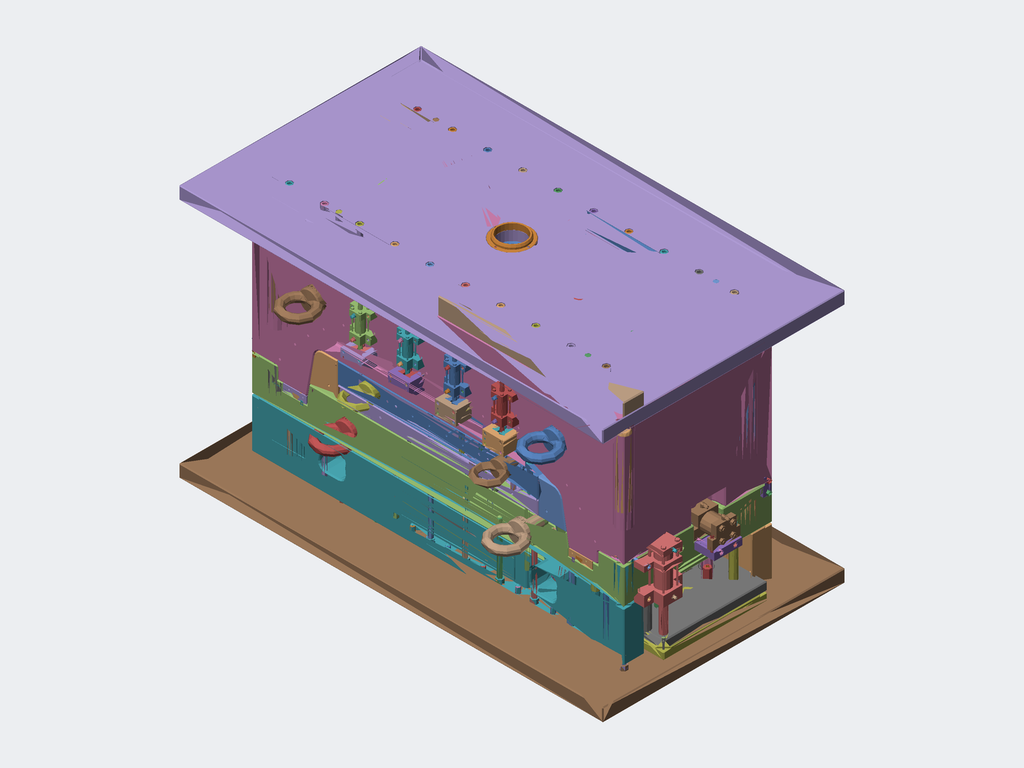Assembly | STEP file | 249 different items | 1127 placed
Parts list (item | name | quantity | parent item | size | volume):
1 | solid 1 | x44 | in A3 | 16 x 16 x 65 mm | 6021 mm3
2 | solid 10 | x4 | in A3 | 40 x 40 x 100 mm | 109109 mm3
3 | solid 100 | x2 | in A3 | 141 x 24 x 24 mm | 30892 mm3
4 | solid 101 | x4 | in A3 | 18 x 18 x 82 mm | 10396 mm3
5 | solid 102 | x1 | in A3 | 80 x 100 x 40 mm | 232410 mm3
6 | solid 103 | x1 | in A3 | 10 x 24 x 10 mm | 907.17 mm3
7 | solid 104 | x2 | in A3 | 30 x 112.165 x 452.721 mm | 308363 mm3
8 | solid 105 | x1 | in A3 | 169 x 36 x 36 mm | 85875 mm3
9 | solid 106 | x1 | in A3 | 2450 x 1400 x 75.5 mm | 255795045 mm3
10 | solid 107 | x1 | in A3 | 1075 x 120 x 100 mm | 12371190 mm3
11 | solid 108 | x1 | in A3 | 1075 x 120.001 x 100 mm | 10949894 mm3
12 | solid 109 | x20 | in A3 | 36 x 36 x 209.5 mm | 104197 mm3
13 | solid 11 | x4 | in A3 | 40 x 40 x 100 mm | 109109 mm3
14 | solid 110 | x4 | in A3 | 30 x 30 x 140 mm | 98871 mm3
15 | solid 111 | x1 | in A3 | 14.856 x 17.662 x 17.662 mm | 2886 mm3
16 | solid 112 | x1 | in A3 | 14.856 x 17.662 x 17.662 mm | 2886 mm3
17 | solid 113 | x3 | in A3 | 15.066 x 16.653 x 17.055 mm | 1616 mm3
18 | solid 114 | x2 | in A3 | 18.126 x 15.123 x 18.251 mm | 1616 mm3
19 | solid 115 | x4 | in A3 | 16 x 16 x 38 mm | 3900 mm3
20 | solid 116 | x1 | in A3 | 100 x 25.292 x 82.969 mm | 104423 mm3
21 | solid 117 | x6 | in A3 | 23.471 x 100 x 70 mm | 88768 mm3
22 | solid 118 | x2 | in A3 | 64.193 x 74.193 x 40 mm | 137435 mm3
23 | solid 119 | x16 | in A3 | 16 x 16 x 54 mm | 5157 mm3
24 | solid 12 | x20 | in A3 | 36 x 36 x 324 mm | 155996 mm3
25 | solid 120 | x1 | in A3 | 25 x 36.961 x 150.435 mm | 48566 mm3
26 | solid 121 | x1 | in A3 | 20 x 20 x 674.011 mm | 136324 mm3
27 | solid 122 | x1 | in A3 | - | 271064204 mm3
28 | solid 123 | x1 | in A3 | 25 x 36.961 x 150.435 mm | 48566 mm3
29 | solid 124 | x2 | in A3 | 120 x 30.646 x 121.053 mm | 166220 mm3
30 | solid 125 | x1 | in A3 | 20 x 20 x 674.011 mm | 136325 mm3
31 | solid 126 | x1 | in A3 | 275.799 x 860 x 518.917 mm | 54222779 mm3
32 | solid 127 | x1 | in A3 | 215.526 x 420.609 x 290.404 mm | 6486474 mm3
33 | solid 128 | x1 | in A3 | 1159 x 120 x 150 mm | 11583265 mm3
34 | solid 129 | x12 | in A3 | 36 x 36 x 114 mm | 60994 mm3
35 | solid 13 | x2 | in A3 | 98 x 98 x 290 mm | 2182712 mm3
36 | solid 130 | x2 | in A3 | 100 x 100 x 80 mm | 601369 mm3
37 | solid 131 | x2 | in A3 | 24 x 24 x 103 mm | 23254 mm3
38 | solid 132 | x4 | in A3 | 45 x 45 x 440 mm | 555891 mm3
39 | solid 133 | x24 | in A3 | 34 x 17 x 19.63 mm | 5633 mm3
40 | solid 134 | x4 | in A3 | 81 x 24 x 24 mm | 18829 mm3
41 | solid 135 | x1 | in A3 | 115 x 220 x 470 mm | 3142718 mm3
42 | solid 136 | x4 | in A3 | 18 x 18 x 77 mm | 9833 mm3
43 | solid 137 | x4 | in A3 | 40 x 40 x 60 mm | 64101 mm3
44 | solid 138 | x8 | in A3 | 36 x 36 x 154 mm | 79089 mm3
45 | solid 139 | x1 | in A3 | 169 x 36 x 36 mm | 85875 mm3
46 | solid 14 | x5 | in A3 | 18 x 18 x 67 mm | 8702 mm3
47 | solid 140 | x1 | in A3 | 119 x 36 x 36 mm | 63256 mm3
48 | solid 141 | x2 | in A3 | 166 x 236 x 100.5 mm | 770612 mm3
49 | solid 142 | x2 | in A3 | 166 x 236 x 100.5 mm | 770612 mm3
50 | solid 143 | x4 | in A3 | 70 x 60 x 80 mm | 220295 mm3
51 | solid 144 | x2 | in A3 | 120 x 90 x 80 mm | 514851 mm3
52 | solid 145 | x4 | in A3 | 25 x 214.479 x 25 mm | 62211 mm3
53 | solid 146 | x4 | in A3 | 10 x 100 x 10 mm | 7854 mm3
54 | solid 147 | x8 | in A3 | 16 x 50 x 16 mm | 4838 mm3
55 | solid 148 | x1 | in A3 | 120 x 70 x 261 mm | 645284 mm3
56 | solid 149 | x4 | in A3 | 16 x 120 x 16 mm | 24127 mm3
57 | solid 15 | x1 | in A3 | 2450 x 1400 x 75.5 mm | 249798342 mm3
58 | solid 150 | x4 | in A3 | 25 x 210.948 x 25 mm | 49531 mm3
59 | solid 151 | x1 | in A3 | 335.969 x 60 x 260.545 mm | 1623800 mm3
60 | solid 152 | x2 | in A3 | 400.456 x 100 x 296.842 mm | 2354176 mm3
61 | solid 153 | x1 | in A3 | 191.822 x 70 x 220.454 mm | 648426 mm3
62 | solid 154 | x2 | in A3 | 25 x 212.652 x 25 mm | 69526 mm3
63 | solid 155 | x2 | in A3 | 25 x 214.101 x 25 mm | 62890 mm3
64 | solid 156 | x4 | in A3 | 18 x 57 x 18 mm | 7569 mm3
65 | solid 157 | x2 | in A3 | 209.196 x 80 x 256.267 mm | 975283 mm3
66 | solid 158 | x6 | in A3 | 33.249 x 33.249 x 28.575 mm | 19000 mm3
67 | solid 159 | x5 | in A3 | 33.249 x 33.249 x 28.575 mm | 19000 mm3
68 | solid 16 | x37 | in A3 | 17.662 x 14.856 x 17.662 mm | 2886 mm3
69 | solid 160 | x1 | in A3 | 30.5 x 1 x 274.425 mm | 8203 mm3
70 | solid 161 | x6 | in A3 | 30.5 x 30.5 x 309.163 mm | 221417 mm3
71 | solid 162 | x1 | in A3 | 30.5 x 1 x 214.425 mm | 6372 mm3
72 | solid 163 | x1 | in A3 | 30.5 x 1 x 159.425 mm | 4694 mm3
73 | solid 164 | x1 | in A3 | 30.5 x 1 x 144.425 mm | 4236 mm3
74 | solid 165 | x1 | in A3 | 30.5 x 1 x 134.425 mm | 3931 mm3
75 | solid 166 | x1 | in A3 | 30.5 x 1 x 129.425 mm | 3778 mm3
76 | solid 167 | x12 | in A3 | 33.249 x 33.249 x 28.575 mm | 19000 mm3
77 | solid 168 | x5 | in A3 | 33.249 x 33.249 x 28.575 mm | 19000 mm3
78 | solid 169 | x4 | in A3 | 15 x 240 x 15 mm | 42412 mm3
79 | solid 17 | x8 | in A3 | 28.401 x 28.401 x 2.4 mm | 543.953 mm3
80 | solid 170 | x16 | in A3 | 16 x 50 x 16 mm | 4838 mm3
81 | solid 171 | x2 | in A3 | 120 x 70 x 281 mm | 651567 mm3
82 | solid 172 | x4 | in A3 | 10 x 10 x 21 mm | 822.37 mm3
83 | solid 173 | x5 | in A3 | 30 x 30 x 13 mm | 8174 mm3
84 | solid 174 | x4 | in A3 | 16 x 16 x 30 mm | 6011 mm3
85 | solid 175 | x4 | in A3 | 30 x 30 x 10 mm | 4966 mm3
86 | solid 176 | x4 | in A3 | 18 x 57 x 18 mm | 7569 mm3
87 | solid 177 | x2 | in A3 | 120 x 70 x 271 mm | 648426 mm3
88 | solid 178 | x8 | in A3 | 16 x 50 x 16 mm | 4838 mm3
89 | solid 179 | x1 | in A3 | 120 x 70 x 261 mm | 645284 mm3
90 | solid 18 | x5 | in A3 | 36 x 36 x 119 mm | 63256 mm3
91 | solid 180 | x1 | in A3 | 191.822 x 70 x 220.454 mm | 648426 mm3
92 | solid 181 | x1 | in A3 | 166.33 x 90 x 157.702 mm | 730851 mm3
93 | solid 182 | x1 | in A3 | 335.969 x 60 x 260.545 mm | 1623800 mm3
94 | solid 183 | x16 | in A3 | 16 x 104.2 x 16 mm | 9078 mm3
95 | solid 184 | x4 | in A3 | 70 x 60 x 80 mm | 220295 mm3
96 | solid 185 | x4 | in A3 | 120 x 90 x 80 mm | 514851 mm3
97 | solid 186 | x1 | in A3 | 78 x 78 x 172.328 mm | 163780 mm3
98 | solid 187 | x2 | in A3 | 25 x 204.048 x 25 mm | 59820 mm3
99 | solid 188 | x2 | in A3 | 25 x 209.468 x 25 mm | 61087 mm3
100 | solid 189 | x1 | in A3 | 78 x 78 x 380.197 mm | 321503 mm3
101 | solid 19 | x2 | in A3 | 13 x 13 x 31 mm | 2077 mm3
102 | solid 190 | x18 | in A3 | 33.249 x 33.249 x 28.575 mm | 19000 mm3
103 | solid 191 | x18 | in A3 | 33.249 x 33.249 x 28.575 mm | 19000 mm3
104 | solid 192 | x1 | in A3 | 33.249 x 33.249 x 28.575 mm | 19000 mm3
105 | solid 193 | x2 | in A3 | 102 x 14 x 16.166 mm | 8632 mm3
106 | solid 194 | x4 | in A3 | 81 x 24 x 24 mm | 18829 mm3
107 | solid 195 | x10 | in A3 | 13 x 13 x 103 mm | 5695 mm3
108 | solid 196 | x2 | in A3 | 28.652 x 26.452 x 20 mm | 5174 mm3
109 | solid 197 | x2 | in A3 | 26.803 x 29.047 x 24 mm | 6695 mm3
110 | solid 198 | x2 | in A3 | 78 x 78 x 475.57 mm | 368550 mm3
111 | solid 199 | x4 | in A3 | 12.786 x 19.739 x 20 mm | 475.009 mm3
112 | solid 2 | x2 | in A3 | 98 x 98 x 290 mm | 2182712 mm3
113 | solid 20 | x2 | in A3 | 99.984 x 40 x 48.51 mm | 156692 mm3
114 | solid 200 | x2 | in A3 | 28.652 x 26.452 x 20 mm | 5174 mm3
115 | solid 201 | x2 | in A3 | 26.803 x 29.047 x 24 mm | 6695 mm3
116 | solid 202 | x2 | in A3 | 13 x 13 x 98 mm | 5444 mm3
117 | solid 203 | x1 | in A3 | 10 x 24 x 10 mm | 907.171 mm3
118 | solid 204 | x2 | in A3 | 141 x 24 x 24 mm | 30892 mm3
119 | solid 205 | x1 | in A3 | 115 x 160 x 40 mm | 667851 mm3
120 | solid 206 | x1 | in A3 | 320.319 x 160 x 137.691 mm | 2188170 mm3
121 | solid 207 | x4 | in A3 | 42 x 42 x 12 mm | 15756 mm3
122 | solid 208 | x4 | in A3 | 10 x 10 x 21 mm | 822.719 mm3
123 | solid 209 | x12 | in A3 | 10 x 10 x 19 mm | 766.17 mm3
124 | solid 21 | x9 | in A3 | 17.662 x 17.662 x 14.856 mm | 2886 mm3
125 | solid 210 | x4 | in A3 | 125 x 125 x 10 mm | 67442 mm3
126 | solid 211 | x4 | in A3 | 95 x 95 x 120 mm | 243778 mm3
127 | solid 212 | x1 | in A3 | 2150 x 860 x 210.001 mm | 305924028 mm3
128 | solid 213 | x1 | in A3 | 115 x 220 x 470 mm | 3142718 mm3
129 | solid 214 | x2 | in A3 | 45 x 52.5 x 46 mm | 85031 mm3
130 | solid 215 | x2 | in A3 | 68 x 24 x 24 mm | 16217 mm3
131 | solid 216 | x2 | in A3 | 70 x 65 x 18 mm | 70637 mm3
132 | solid 217 | x2 | in A3 | 120 x 65 x 18 mm | 129137 mm3
133 | solid 218 | x1 | in A3 | 10 x 24 x 10 mm | 907.171 mm3
134 | solid 219 | x2 | in A3 | 15 x 15 x 25 mm | 4386 mm3
135 | solid 22 | x2 | in A3 | 121.532 x 24.876 x 80 mm | 116975 mm3
136 | solid 220 | x1 | in A3 | 10 x 24 x 10 mm | 907.17 mm3
137 | solid 221 | x3 | in A3 | 30 x 73.163 x 849.352 mm | 585466 mm3
138 | solid 222 | x4 | in A3 | 101 x 100 x 60 mm | 261945 mm3
139 | solid 223 | x8 | in A3 | 30 x 30 x 30 mm | 9761 mm3
140 | solid 224 | x1 | in A3 | 645.466 x 105.916 x 113.789 mm | 5298019 mm3
141 | solid 225 | x1 | in A3 | 80 x 100 x 40 mm | 232410 mm3
142 | solid 226 | x1 | in A3 | 2350 x 620 x 50 mm | 60712018 mm3
143 | solid 227 | x1 | in A3 | 2350 x 620 x 50 mm | 65620843 mm3
144 | solid 228 | x1 | in A3 | 2150 x 120 x 290 mm | 66813400 mm3
145 | solid 229 | x1 | in A3 | 2150 x 120 x 290 mm | 67733928 mm3
146 | solid 23 | x1 | in A3 | 135.51 x 264.332 x 188.118 mm | 3455186 mm3
147 | solid 230 | x4 | in A3 | 13 x 13 x 26 mm | 1825 mm3
148 | solid 231 | x1 | in A3 | 175 x 175 x 20 mm | 232149 mm3
149 | solid 232 | x1 | in A3 | 210 x 210 x 35 mm | 357720 mm3
150 | solid 233 | x1 | in A3 | 1344 x 458.517 x 80 mm | 15931765 mm3
151 | solid 234 | x1 | in A3 | 10 x 10 x 21 mm | 822.37 mm3
152 | solid 235 | x4 | in A3 | 13 x 13 x 103 mm | 5695 mm3
153 | solid 236 | x2 | in A3 | 22 x 22 x 728.65 mm | 268884 mm3
154 | solid 237 | x1 | in A3 | 1075 x 120 x 100 mm | 12067312 mm3
155 | solid 238 | x1 | in A3 | 1075 x 120 x 100 mm | 10949620 mm3
156 | solid 239 | x1 | in A3 | 1159 x 120 x 150 mm | 11582986 mm3
157 | solid 24 | x6 | in A3 | 14.157 x 12.856 x 14.157 mm | 1616 mm3
158 | solid 240 | x2 | in A3 | 22 x 22 x 730.955 mm | 269760 mm3
159 | solid 241 | x1 | in A3 | 74.217 x 43.029 x 40.25 mm | 106174 mm3
160 | solid 242 | x2 | in A3 | 74.238 x 44.192 x 40.9 mm | 109549 mm3
161 | solid 243 | x1 | in A3 | 74.214 x 43.098 x 40.392 mm | 106427 mm3
162 | solid 244 | x2 | in A3 | 94.183 x 59.188 x 39.916 mm | 147837 mm3
163 | solid 245 | x1 | in A3 | 35 x 46.15 x 148.499 mm | 104448 mm3
164 | solid 246 | x2 | in A3 | 40 x 85.054 x 24 mm | 60155 mm3
165 | solid 247 | x1 | in A3 | 35 x 46.15 x 148.499 mm | 104448 mm3
166 | solid 248 | x1 | in A3 | 819.765 x 65.53 x 111.578 mm | 4185351 mm3
167 | solid 249 | x1 | in A3 | - | -
168 | solid 25 | x8 | in A3 | 14.157 x 12.856 x 14.157 mm | 1616 mm3
169 | solid 26 | x1 | in A3 | 135.51 x 264.332 x 188.118 mm | 3455192 mm3
170 | solid 27 | x2 | in A3 | 11.3 x 11.3 x 16.5 mm | 595.104 mm3
171 | solid 28 | x2 | in A3 | 32 x 32 x 8 mm | 5898 mm3
172 | solid 29 | x2 | in A3 | 35 x 35 x 965 mm | 683981 mm3
173 | solid 3 | x4 | in A3 | 24 x 24 x 86.5 mm | 19937 mm3
174 | solid 30 | x12 | in A3 | 10 x 110 x 10 mm | 8639 mm3
175 | solid 31 | x8 | in A3 | 16 x 104.2 x 16 mm | 9078 mm3
176 | solid 32 | x1 | in A3 | 166.33 x 90 x 157.702 mm | 730851 mm3
177 | solid 33 | x8 | in A3 | 16 x 104.2 x 16 mm | 9078 mm3
178 | solid 34 | x2 | in A3 | 25.029 x 60 x 25.037 mm | 10130 mm3
179 | solid 35 | x3 | in A3 | 25.029 x 50 x 25.037 mm | 8248 mm3
180 | solid 36 | x2 | in A3 | 56 x 24 x 24 mm | 13802 mm3
181 | solid 37 | x2 | in A3 | 15 x 50 x 100 mm | 66748 mm3
182 | solid 38 | x2 | in A3 | 56 x 24 x 24 mm | 13802 mm3
183 | solid 39 | x4 | in A3 | 70 x 70 x 435 mm | 1546175 mm3
184 | solid 4 | x4 | in A3 | 50 x 50 x 360 mm | 617922 mm3
185 | solid 40 | x4 | in A3 | 90 x 90 x 422 mm | 2099670 mm3
186 | solid 41 | x1 | in A3 | 164.037 x 503.365 x 295.607 mm | 9582610 mm3
187 | solid 42 | x1 | in A3 | 164.037 x 503.365 x 295.607 mm | 9580661 mm3
188 | solid 43 | x1 | in A3 | - | -
189 | solid 44 | x4 | in A3 | 206 x 298 x 120.501 mm | 1511005 mm3
190 | solid 45 | x4 | in A3 | 206 x 298 x 120.501 mm | 1511009 mm3
191 | solid 46 | x1 | in A3 | - | 211233 mm3
192 | solid 47 | x2 | in A3 | 32 x 32 x 30 mm | 9356 mm3
193 | solid 48 | x1 | in A3 | 25 x 25 x 917.392 mm | 438618 mm3
194 | solid 49 | x4 | in A3 | 100 x 100 x 100 mm | 753638 mm3
195 | solid 5 | x4 | in A3 | 70 x 70 x 100 mm | 136102 mm3
196 | solid 50 | x20 | in A3 | 24 x 24 x 123 mm | 27276 mm3
197 | solid 51 | x2 | in A3 | 120 x 120 x 18 mm | 247072 mm3
198 | solid 52 | x2 | in A3 | 110 x 100 x 18 mm | 185872 mm3
199 | solid 53 | x40 | in A3 | 13 x 13 x 29 mm | 1976 mm3
200 | solid 54 | x2 | in A3 | 185 x 100 x 18 mm | 283727 mm3
201 | solid 55 | x2 | in A3 | 120 x 34.962 x 151.763 mm | 223888 mm3
202 | solid 56 | x1 | in A3 | 120 x 27.824 x 103.411 mm | 144143 mm3
203 | solid 57 | x1 | in A3 | 120 x 34.115 x 145.737 mm | 224584 mm3
204 | solid 58 | x1 | in A3 | 120 x 27.859 x 104.131 mm | 135753 mm3
205 | solid 59 | x4 | in A3 | 30 x 30 x 215.5 mm | 152239 mm3
206 | solid 6 | x24 | in A3 | 30 x 30 x 10 mm | 6388 mm3
207 | solid 60 | x1 | in A3 | 16 x 14 x 783.319 mm | 88933 mm3
208 | solid 61 | x1 | in A3 | 215.526 x 420.609 x 290.404 mm | 6488252 mm3
209 | solid 62 | x1 | in A3 | 275.804 x 860 x 518.917 mm | 54217917 mm3
210 | solid 63 | x2 | in A3 | 414.488 x 213.171 x 497.487 mm | 6813451 mm3
211 | solid 64 | x9 | in A3 | 49.314 x 40 x 57.016 mm | 27434 mm3
212 | solid 65 | x5 | in A3 | 14.157 x 14.157 x 12.856 mm | 1616 mm3
213 | solid 66 | x8 | in A3 | 36 x 36 x 134 mm | 70042 mm3
214 | solid 67 | x22 | in A3 | 60 x 11 x 35 mm | 20301 mm3
215 | solid 68 | x44 | in A3 | 18 x 18 x 57 mm | 7571 mm3
216 | solid 69 | x4 | in A3 | 18.126 x 15.123 x 18.251 mm | 1616 mm3
217 | solid 7 | x24 | in A3 | 11.3 x 11.3 x 19.7 mm | 685.582 mm3
218 | solid 70 | x2 | in A3 | 17.662 x 17.662 x 14.856 mm | 2886 mm3
219 | solid 71 | x4 | in A3 | 16 x 16 x 36 mm | 3743 mm3
220 | solid 72 | x22 | in A3 | 10 x 10 x 40 mm | 2932 mm3
221 | solid 73 | x2 | in A3 | 68 x 24 x 24 mm | 16217 mm3
222 | solid 74 | x2 | in A3 | 45 x 52.5 x 46 mm | 85031 mm3
223 | solid 75 | x3 | in A3 | 15.066 x 16.653 x 17.055 mm | 1616 mm3
224 | solid 76 | x4 | in A3 | 10 x 10 x 40 mm | 2931 mm3
225 | solid 77 | x8 | in A3 | 16 x 16 x 44 mm | 4371 mm3
226 | solid 78 | x2 | in A3 | 35.54 x 80 x 162.326 mm | 129819 mm3
227 | solid 79 | x11 | in A3 | 22.76 x 18 x 42.786 mm | 5761 mm3
228 | solid 8 | x22 | in A3 | 24 x 24 x 73 mm | 17222 mm3
229 | solid 80 | x1 | in A3 | 33.249 x 33.249 x 28.575 mm | 19000 mm3
230 | solid 81 | x9 | in A3 | 100 x 80 x 40 mm | 256419 mm3
231 | solid 82 | x2 | in A3 | 102 x 14 x 16.166 mm | 8632 mm3
232 | solid 83 | x2 | in A3 | 40 x 54.339 x 85.972 mm | 43927 mm3
233 | solid 84 | x2 | in A3 | 17.662 x 17.662 x 14.856 mm | 2886 mm3
234 | solid 85 | x6 | in A3 | 60 x 56.714 x 56.714 mm | 73718 mm3
235 | solid 86 | x2 | in A3 | 15 x 15 x 25 mm | 4386 mm3
236 | solid 87 | x7 | in A3 | 101 x 100 x 60 mm | 261945 mm3
237 | solid 88 | x2 | in A3 | 165.903 x 35 x 30 mm | 145884 mm3
238 | solid 89 | x2 | in A3 | 163.329 x 46.356 x 30 mm | 173542 mm3
239 | solid 9 | x22 | in A3 | 36 x 36 x 109.5 mm | 58958 mm3
240 | solid 90 | x1 | in A3 | 14.856 x 17.662 x 17.662 mm | 2886 mm3
241 | solid 91 | x1 | in A3 | 14.856 x 17.662 x 17.662 mm | 2886 mm3
242 | solid 92 | x2 | in A3 | 30 x 159.47 x 696.084 mm | 483606 mm3
243 | solid 93 | x5 | in A3 | 57.224 x 60 x 57.224 mm | 73718 mm3
244 | solid 94 | x4 | in A3 | 29.965 x 100 x 117.263 mm | 138238 mm3
245 | solid 95 | x4 | in A3 | 137.91 x 30 x 538.185 mm | 371040 mm3
246 | solid 96 | x2 | in A3 | 40 x 193.057 x 22 mm | 131718 mm3
247 | solid 97 | x4 | in A3 | 18 x 18 x 82 mm | 10396 mm3
248 | solid 98 | x1 | in A3 | 115 x 160 x 40 mm | 667851 mm3
249 | solid 99 | x1 | in A3 | 320.319 x 160 x 137.691 mm | 2188173 mm3